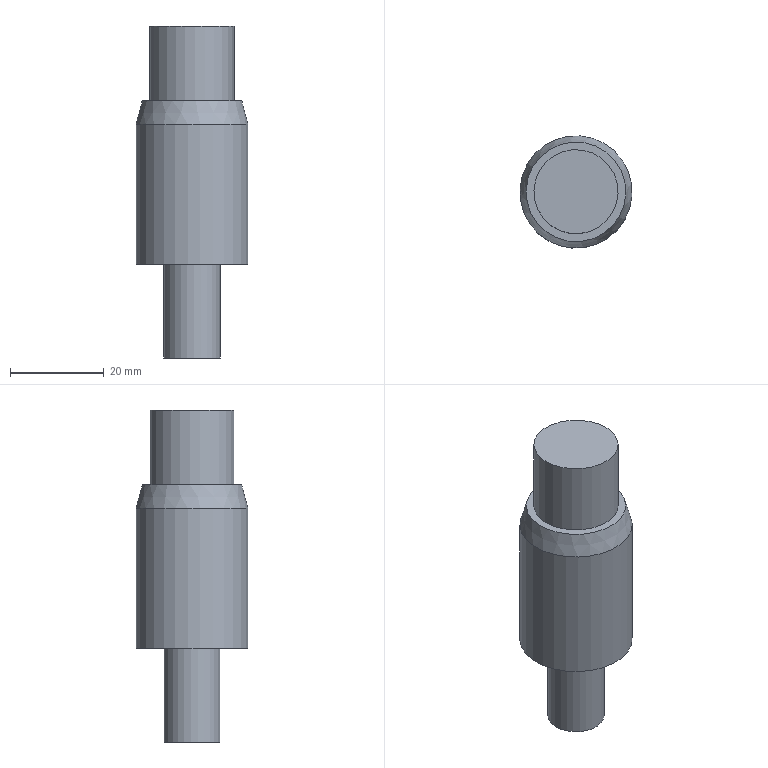Part | NX | features solid 2 | 1 solid | 8 faces | box 24 x 24 x 71 mm | volume 21924 mm3 | plane 4 | cylinder 3 | cone 1 | commonest cylinder face diameters 12 x1 18 x1 24 x1
STEP:
#1=CARTESIAN_POINT('',(1454.608,-649.,20.));
#2=VERTEX_POINT('',#1);
#3=CARTESIAN_POINT('',(1465.,-655.,20.));
#4=DIRECTION('',(0.,0.,-1.));
#5=DIRECTION('',(-0.866,0.5,0.));
#6=AXIS2_PLACEMENT_3D('',#3,#4,#5);
#7=CIRCLE('',#6,12.);
#8=EDGE_CURVE('',#2,#2,#7,.F.);
#9=ORIENTED_EDGE('',*,*,#8,.F.);
#10=EDGE_LOOP('',(#9));
#11=FACE_BOUND('',#10,.T.);
#12=CARTESIAN_POINT('',(1454.608,-649.,-10.));
#13=VERTEX_POINT('',#12);
#14=CARTESIAN_POINT('',(1465.,-655.,-10.));
#15=DIRECTION('',(0.,0.,-1.));
#16=DIRECTION('',(-0.866,0.5,0.));
#17=AXIS2_PLACEMENT_3D('',#14,#15,#16);
#18=CIRCLE('',#17,12.);
#19=EDGE_CURVE('',#13,#13,#18,.T.);
#20=ORIENTED_EDGE('',*,*,#19,.F.);
#21=EDGE_LOOP('',(#20));
#22=FACE_BOUND('',#21,.T.);
#23=CARTESIAN_POINT('',(1465.,-655.,25.));
#24=DIRECTION('',(0.,0.,-1.));
#25=DIRECTION('',(0.866,-0.5,0.));
#26=AXIS2_PLACEMENT_3D('',#23,#24,#25);
#27=CYLINDRICAL_SURFACE('',#26,12.);
#28=ADVANCED_FACE('',(#11,#22),#27,.T.);
#29=CARTESIAN_POINT('',(1457.206,-650.5,25.));
#30=VERTEX_POINT('',#29);
#31=CARTESIAN_POINT('',(1465.,-655.,25.));
#32=DIRECTION('',(0.,0.,-1.));
#33=DIRECTION('',(-0.866,0.5,0.));
#34=AXIS2_PLACEMENT_3D('',#31,#32,#33);
#35=CIRCLE('',#34,9.);
#36=EDGE_CURVE('',#30,#30,#35,.T.);
#37=ORIENTED_EDGE('',*,*,#36,.T.);
#38=EDGE_LOOP('',(#37));
#39=FACE_BOUND('',#38,.T.);
#40=CARTESIAN_POINT('',(1455.768,-649.67,25.));
#41=VERTEX_POINT('',#40);
#42=CARTESIAN_POINT('',(1465.,-655.,25.));
#43=DIRECTION('',(0.,0.,-1.));
#44=DIRECTION('',(-0.866,0.5,0.));
#45=AXIS2_PLACEMENT_3D('',#42,#43,#44);
#46=CIRCLE('',#45,10.66);
#47=EDGE_CURVE('',#41,#41,#46,.T.);
#48=ORIENTED_EDGE('',*,*,#47,.F.);
#49=EDGE_LOOP('',(#48));
#50=FACE_BOUND('',#49,.T.);
#51=CARTESIAN_POINT('',(1465.,-655.,25.));
#52=DIRECTION('',(0.,0.,1.));
#53=DIRECTION('',(-0.866,0.5,0.));
#54=AXIS2_PLACEMENT_3D('',#51,#52,#53);
#55=PLANE('',#54);
#56=ADVANCED_FACE('',(#39,#50),#55,.T.);
#57=CARTESIAN_POINT('',(1470.196,-658.,-10.));
#58=VERTEX_POINT('',#57);
#59=CARTESIAN_POINT('',(1465.,-655.,-10.));
#60=DIRECTION('',(0.,0.,1.));
#61=DIRECTION('',(0.866,-0.5,0.));
#62=AXIS2_PLACEMENT_3D('',#59,#60,#61);
#63=CIRCLE('',#62,6.);
#64=EDGE_CURVE('',#58,#58,#63,.T.);
#65=ORIENTED_EDGE('',*,*,#64,.T.);
#66=EDGE_LOOP('',(#65));
#67=FACE_BOUND('',#66,.T.);
#68=ORIENTED_EDGE('',*,*,#19,.T.);
#69=EDGE_LOOP('',(#68));
#70=FACE_BOUND('',#69,.T.);
#71=CARTESIAN_POINT('',(1465.,-655.,-10.));
#72=DIRECTION('',(0.,0.,1.));
#73=DIRECTION('',(-0.866,0.5,0.));
#74=AXIS2_PLACEMENT_3D('',#71,#72,#73);
#75=PLANE('',#74);
#76=ADVANCED_FACE('',(#67,#70),#75,.F.);
#77=ORIENTED_EDGE('',*,*,#8,.T.);
#78=EDGE_LOOP('',(#77));
#79=FACE_BOUND('',#78,.T.);
#80=ORIENTED_EDGE('',*,*,#47,.T.);
#81=EDGE_LOOP('',(#80));
#82=FACE_BOUND('',#81,.T.);
#83=CARTESIAN_POINT('',(1465.,-655.,25.));
#84=DIRECTION('',(0.,0.,-1.));
#85=DIRECTION('',(0.866,-0.5,0.));
#86=AXIS2_PLACEMENT_3D('',#83,#84,#85);
#87=CONICAL_SURFACE('',#86,10.66,0.2618);
#88=ADVANCED_FACE('',(#79,#82),#87,.T.);
#89=CARTESIAN_POINT('',(1470.196,-658.,-30.));
#90=VERTEX_POINT('',#89);
#91=CARTESIAN_POINT('',(1465.,-655.,-30.));
#92=DIRECTION('',(0.,0.,1.));
#93=DIRECTION('',(0.866,-0.5,0.));
#94=AXIS2_PLACEMENT_3D('',#91,#92,#93);
#95=CIRCLE('',#94,6.);
#96=EDGE_CURVE('',#90,#90,#95,.T.);
#97=ORIENTED_EDGE('',*,*,#96,.F.);
#98=EDGE_LOOP('',(#97));
#99=FACE_BOUND('',#98,.T.);
#100=CARTESIAN_POINT('',(1465.,-655.,-30.));
#101=DIRECTION('',(0.,0.,-1.));
#102=DIRECTION('',(0.866,-0.5,0.));
#103=AXIS2_PLACEMENT_3D('',#100,#101,#102);
#104=PLANE('',#103);
#105=ADVANCED_FACE('',(#99),#104,.T.);
#106=ORIENTED_EDGE('',*,*,#96,.T.);
#107=EDGE_LOOP('',(#106));
#108=FACE_BOUND('',#107,.T.);
#109=ORIENTED_EDGE('',*,*,#64,.F.);
#110=EDGE_LOOP('',(#109));
#111=FACE_BOUND('',#110,.T.);
#112=CARTESIAN_POINT('',(1465.,-655.,-10.));
#113=DIRECTION('',(0.,0.,-1.));
#114=DIRECTION('',(0.866,-0.5,0.));
#115=AXIS2_PLACEMENT_3D('',#112,#113,#114);
#116=CYLINDRICAL_SURFACE('',#115,6.);
#117=ADVANCED_FACE('',(#108,#111),#116,.T.);
#118=CARTESIAN_POINT('',(1457.206,-650.5,41.));
#119=VERTEX_POINT('',#118);
#120=CARTESIAN_POINT('',(1465.,-655.,41.));
#121=DIRECTION('',(0.,0.,-1.));
#122=DIRECTION('',(-0.866,0.5,0.));
#123=AXIS2_PLACEMENT_3D('',#120,#121,#122);
#124=CIRCLE('',#123,9.);
#125=EDGE_CURVE('',#119,#119,#124,.T.);
#126=ORIENTED_EDGE('',*,*,#125,.F.);
#127=EDGE_LOOP('',(#126));
#128=FACE_BOUND('',#127,.T.);
#129=CARTESIAN_POINT('',(1465.,-655.,41.));
#130=DIRECTION('',(0.,0.,1.));
#131=DIRECTION('',(-0.866,0.5,0.));
#132=AXIS2_PLACEMENT_3D('',#129,#130,#131);
#133=PLANE('',#132);
#134=ADVANCED_FACE('',(#128),#133,.T.);
#135=ORIENTED_EDGE('',*,*,#125,.T.);
#136=EDGE_LOOP('',(#135));
#137=FACE_BOUND('',#136,.T.);
#138=ORIENTED_EDGE('',*,*,#36,.F.);
#139=EDGE_LOOP('',(#138));
#140=FACE_BOUND('',#139,.T.);
#141=CARTESIAN_POINT('',(1465.,-655.,25.));
#142=DIRECTION('',(0.,0.,1.));
#143=DIRECTION('',(-0.866,0.5,0.));
#144=AXIS2_PLACEMENT_3D('',#141,#142,#143);
#145=CYLINDRICAL_SURFACE('',#144,9.);
#146=ADVANCED_FACE('',(#137,#140),#145,.T.);
#147=CLOSED_SHELL('',(#28,#56,#76,#88,#105,#117,#134,#146));
#148=MANIFOLD_SOLID_BREP('',#147);
#149=(LENGTH_UNIT()NAMED_UNIT(*)SI_UNIT(.MILLI.,.METRE.));
#150=UNCERTAINTY_MEASURE_WITH_UNIT(LENGTH_MEASURE(0.00001),#149,'','');
#151=(NAMED_UNIT(*)PLANE_ANGLE_UNIT()SI_UNIT($,.RADIAN.));
#152=(NAMED_UNIT(*)SI_UNIT($,.STERADIAN.)SOLID_ANGLE_UNIT());
#153=(GEOMETRIC_REPRESENTATION_CONTEXT(3)GLOBAL_UNCERTAINTY_ASSIGNED_CONTEXT((#150))GLOBAL_UNIT_ASSIGNED_CONTEXT((#149,#151,#152))REPRESENTATION_CONTEXT('',''));
#154=ADVANCED_BREP_SHAPE_REPRESENTATION('',(#148),#153);